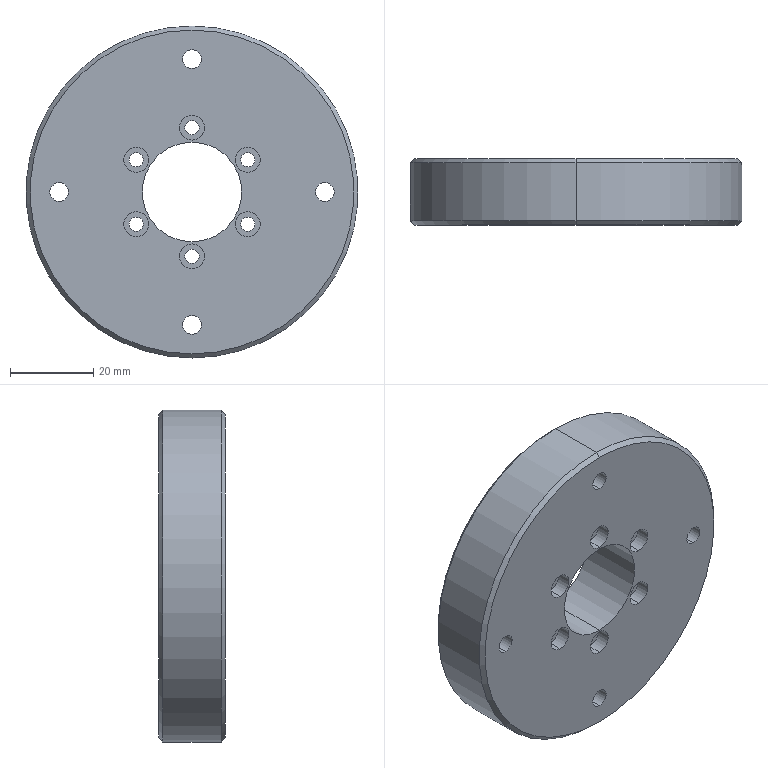Part | SolidWorks | features HoleWzd 2, Chamfer 1, CirPattern 1, Extrusion 1, SketchPattern 1 | 1 solid | 60 faces | box 80 x 16 x 80 mm | volume 70024 mm3 | cylinder 44 | plane 12 | cone 4 | commonest cylinder face diameters 3.4 x12 6 x12 4.5 x8 8 x8 24 x2 80 x2